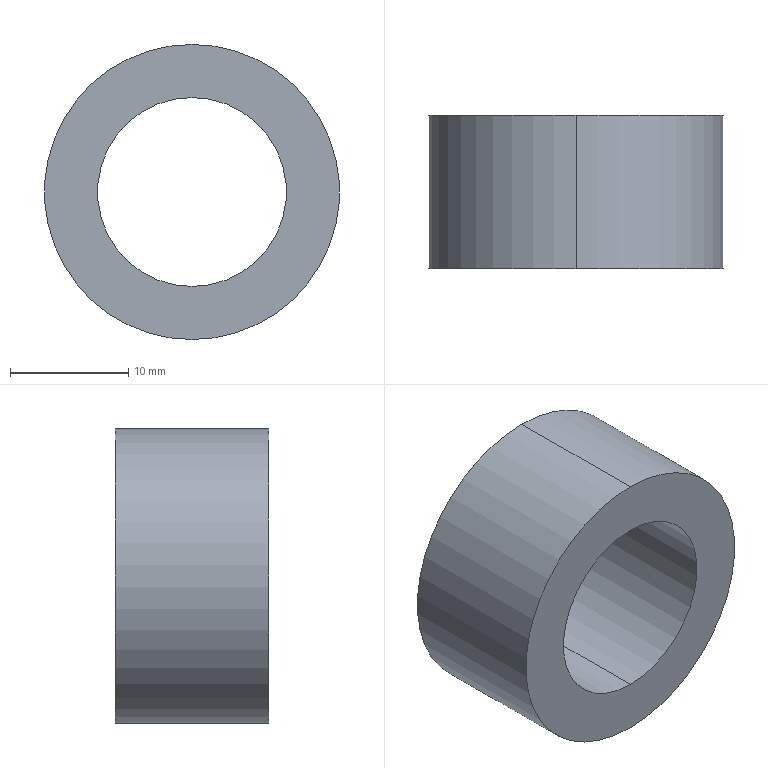Part | SolidWorks | features Extrusion 1 | 1 solid | 6 faces | box 25 x 13 x 25 mm | volume 3768 mm3 | cylinder 4 | plane 2 | commonest cylinder face diameters 16 x2 25 x2
STEP:
#1=CARTESIAN_POINT('',(0.,13.,-8.));
#2=VERTEX_POINT('',#1);
#3=CARTESIAN_POINT('',(0.,13.,8.));
#4=VERTEX_POINT('',#3);
#5=CARTESIAN_POINT('',(0.,13.,0.));
#6=DIRECTION('',(0.,1.,0.));
#7=DIRECTION('',(0.,0.,1.));
#8=AXIS2_PLACEMENT_3D('',#5,#6,#7);
#9=CIRCLE('',#8,8.);
#10=EDGE_CURVE('',#2,#4,#9,.T.);
#11=ORIENTED_EDGE('',*,*,#10,.T.);
#12=CARTESIAN_POINT('',(0.,0.,8.));
#13=VERTEX_POINT('',#12);
#14=CARTESIAN_POINT('',(0.,13.,8.));
#15=DIRECTION('',(0.,-1.,0.));
#16=VECTOR('',#15,1000.);
#17=LINE('',#14,#16);
#18=EDGE_CURVE('',#4,#13,#17,.T.);
#19=ORIENTED_EDGE('',*,*,#18,.T.);
#20=CARTESIAN_POINT('',(0.,0.,-8.));
#21=VERTEX_POINT('',#20);
#22=CARTESIAN_POINT('',(0.,0.,0.));
#23=DIRECTION('',(0.,1.,0.));
#24=DIRECTION('',(0.,0.,1.));
#25=AXIS2_PLACEMENT_3D('',#22,#23,#24);
#26=CIRCLE('',#25,8.);
#27=EDGE_CURVE('',#21,#13,#26,.T.);
#28=ORIENTED_EDGE('',*,*,#27,.F.);
#29=CARTESIAN_POINT('',(0.,13.,-8.));
#30=DIRECTION('',(0.,-1.,0.));
#31=VECTOR('',#30,1000.);
#32=LINE('',#29,#31);
#33=EDGE_CURVE('',#2,#21,#32,.T.);
#34=ORIENTED_EDGE('',*,*,#33,.F.);
#35=EDGE_LOOP('',(#11,#19,#28,#34));
#36=FACE_OUTER_BOUND('',#35,.T.);
#37=CARTESIAN_POINT('',(0.,13.,0.));
#38=DIRECTION('',(0.,-1.,0.));
#39=DIRECTION('',(0.,0.,-1.));
#40=AXIS2_PLACEMENT_3D('',#37,#38,#39);
#41=CYLINDRICAL_SURFACE('',#40,8.);
#42=ADVANCED_FACE('',(#36),#41,.F.);
#43=CARTESIAN_POINT('',(0.,13.,12.5));
#44=VERTEX_POINT('',#43);
#45=CARTESIAN_POINT('',(0.,13.,-12.5));
#46=VERTEX_POINT('',#45);
#47=CARTESIAN_POINT('',(0.,13.,0.));
#48=DIRECTION('',(0.,1.,0.));
#49=DIRECTION('',(0.,0.,1.));
#50=AXIS2_PLACEMENT_3D('',#47,#48,#49);
#51=CIRCLE('',#50,12.5);
#52=EDGE_CURVE('',#44,#46,#51,.T.);
#53=ORIENTED_EDGE('',*,*,#52,.F.);
#54=CARTESIAN_POINT('',(0.,0.,12.5));
#55=VERTEX_POINT('',#54);
#56=CARTESIAN_POINT('',(0.,13.,12.5));
#57=DIRECTION('',(0.,-1.,0.));
#58=VECTOR('',#57,1000.);
#59=LINE('',#56,#58);
#60=EDGE_CURVE('',#44,#55,#59,.T.);
#61=ORIENTED_EDGE('',*,*,#60,.T.);
#62=CARTESIAN_POINT('',(0.,0.,-12.5));
#63=VERTEX_POINT('',#62);
#64=CARTESIAN_POINT('',(0.,0.,0.));
#65=DIRECTION('',(0.,1.,0.));
#66=DIRECTION('',(0.,0.,1.));
#67=AXIS2_PLACEMENT_3D('',#64,#65,#66);
#68=CIRCLE('',#67,12.5);
#69=EDGE_CURVE('',#55,#63,#68,.T.);
#70=ORIENTED_EDGE('',*,*,#69,.T.);
#71=CARTESIAN_POINT('',(0.,13.,-12.5));
#72=DIRECTION('',(0.,-1.,0.));
#73=VECTOR('',#72,1000.);
#74=LINE('',#71,#73);
#75=EDGE_CURVE('',#46,#63,#74,.T.);
#76=ORIENTED_EDGE('',*,*,#75,.F.);
#77=EDGE_LOOP('',(#53,#61,#70,#76));
#78=FACE_OUTER_BOUND('',#77,.T.);
#79=CARTESIAN_POINT('',(0.,13.,0.));
#80=DIRECTION('',(0.,-1.,0.));
#81=DIRECTION('',(0.,0.,-1.));
#82=AXIS2_PLACEMENT_3D('',#79,#80,#81);
#83=CYLINDRICAL_SURFACE('',#82,12.5);
#84=ADVANCED_FACE('',(#78),#83,.T.);
#85=CARTESIAN_POINT('',(0.,13.,0.));
#86=DIRECTION('',(0.,1.,0.));
#87=DIRECTION('',(0.,0.,1.));
#88=AXIS2_PLACEMENT_3D('',#85,#86,#87);
#89=CIRCLE('',#88,12.5);
#90=EDGE_CURVE('',#46,#44,#89,.T.);
#91=ORIENTED_EDGE('',*,*,#90,.T.);
#92=ORIENTED_EDGE('',*,*,#52,.T.);
#93=EDGE_LOOP('',(#91,#92));
#94=FACE_OUTER_BOUND('',#93,.T.);
#95=ORIENTED_EDGE('',*,*,#10,.F.);
#96=CARTESIAN_POINT('',(0.,13.,0.));
#97=DIRECTION('',(0.,1.,0.));
#98=DIRECTION('',(0.,0.,1.));
#99=AXIS2_PLACEMENT_3D('',#96,#97,#98);
#100=CIRCLE('',#99,8.);
#101=EDGE_CURVE('',#4,#2,#100,.T.);
#102=ORIENTED_EDGE('',*,*,#101,.F.);
#103=EDGE_LOOP('',(#95,#102));
#104=FACE_BOUND('',#103,.T.);
#105=CARTESIAN_POINT('',(0.,13.,0.));
#106=DIRECTION('',(0.,1.,0.));
#107=DIRECTION('',(0.,0.,1.));
#108=AXIS2_PLACEMENT_3D('',#105,#106,#107);
#109=PLANE('',#108);
#110=ADVANCED_FACE('',(#94,#104),#109,.T.);
#111=CARTESIAN_POINT('',(0.,0.,0.));
#112=DIRECTION('',(0.,1.,0.));
#113=DIRECTION('',(0.,0.,1.));
#114=AXIS2_PLACEMENT_3D('',#111,#112,#113);
#115=CIRCLE('',#114,12.5);
#116=EDGE_CURVE('',#63,#55,#115,.T.);
#117=ORIENTED_EDGE('',*,*,#116,.F.);
#118=ORIENTED_EDGE('',*,*,#69,.F.);
#119=EDGE_LOOP('',(#117,#118));
#120=FACE_OUTER_BOUND('',#119,.T.);
#121=ORIENTED_EDGE('',*,*,#27,.T.);
#122=CARTESIAN_POINT('',(0.,0.,0.));
#123=DIRECTION('',(0.,1.,0.));
#124=DIRECTION('',(0.,0.,1.));
#125=AXIS2_PLACEMENT_3D('',#122,#123,#124);
#126=CIRCLE('',#125,8.);
#127=EDGE_CURVE('',#13,#21,#126,.T.);
#128=ORIENTED_EDGE('',*,*,#127,.T.);
#129=EDGE_LOOP('',(#121,#128));
#130=FACE_BOUND('',#129,.T.);
#131=CARTESIAN_POINT('',(0.,0.,0.));
#132=DIRECTION('',(0.,1.,0.));
#133=DIRECTION('',(0.,0.,1.));
#134=AXIS2_PLACEMENT_3D('',#131,#132,#133);
#135=PLANE('',#134);
#136=ADVANCED_FACE('',(#120,#130),#135,.F.);
#137=ORIENTED_EDGE('',*,*,#60,.F.);
#138=ORIENTED_EDGE('',*,*,#90,.F.);
#139=ORIENTED_EDGE('',*,*,#75,.T.);
#140=ORIENTED_EDGE('',*,*,#116,.T.);
#141=EDGE_LOOP('',(#137,#138,#139,#140));
#142=FACE_OUTER_BOUND('',#141,.T.);
#143=CARTESIAN_POINT('',(0.,13.,0.));
#144=DIRECTION('',(0.,-1.,0.));
#145=DIRECTION('',(0.,0.,-1.));
#146=AXIS2_PLACEMENT_3D('',#143,#144,#145);
#147=CYLINDRICAL_SURFACE('',#146,12.5);
#148=ADVANCED_FACE('',(#142),#147,.T.);
#149=ORIENTED_EDGE('',*,*,#18,.F.);
#150=ORIENTED_EDGE('',*,*,#101,.T.);
#151=ORIENTED_EDGE('',*,*,#33,.T.);
#152=ORIENTED_EDGE('',*,*,#127,.F.);
#153=EDGE_LOOP('',(#149,#150,#151,#152));
#154=FACE_OUTER_BOUND('',#153,.T.);
#155=CARTESIAN_POINT('',(0.,13.,0.));
#156=DIRECTION('',(0.,-1.,0.));
#157=DIRECTION('',(0.,0.,-1.));
#158=AXIS2_PLACEMENT_3D('',#155,#156,#157);
#159=CYLINDRICAL_SURFACE('',#158,8.);
#160=ADVANCED_FACE('',(#154),#159,.F.);
#161=CLOSED_SHELL('',(#42,#84,#110,#136,#148,#160));
#162=MANIFOLD_SOLID_BREP('',#161);
#163=CARTESIAN_POINT('',(0.,0.,0.));
#164=DIRECTION('',(0.,0.,1.));
#165=DIRECTION('',(1.,0.,0.));
#166=AXIS2_PLACEMENT_3D('',#163,#164,#165);
#167=(LENGTH_UNIT()NAMED_UNIT(*)SI_UNIT(.MILLI.,.METRE.));
#168=UNCERTAINTY_MEASURE_WITH_UNIT(LENGTH_MEASURE(0.00001),#167,'','');
#169=(NAMED_UNIT(*)PLANE_ANGLE_UNIT()SI_UNIT($,.RADIAN.));
#170=(NAMED_UNIT(*)SI_UNIT($,.STERADIAN.)SOLID_ANGLE_UNIT());
#171=(GEOMETRIC_REPRESENTATION_CONTEXT(3)GLOBAL_UNCERTAINTY_ASSIGNED_CONTEXT((#168))GLOBAL_UNIT_ASSIGNED_CONTEXT((#167,#169,#170))REPRESENTATION_CONTEXT('',''));
#172=ADVANCED_BREP_SHAPE_REPRESENTATION('',(#162,#166),#171);